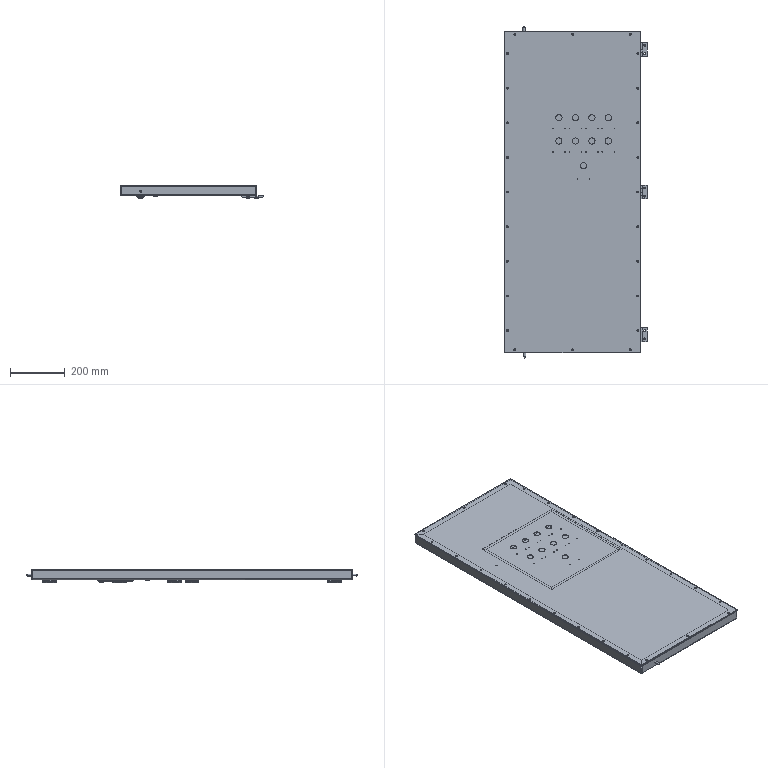Part | SolidWorks | 23 solids | 1907 faces | box 519.5 x 1208 x 50.5 mm | volume 3630200 mm3 | cylinder 839 | plane 765 | spline 226 | cone 69 | torus 8 | commonest cylinder face diameters 1 x144 5 x82 6.1 x70 0.8 x52 6 x52 6.5 x51